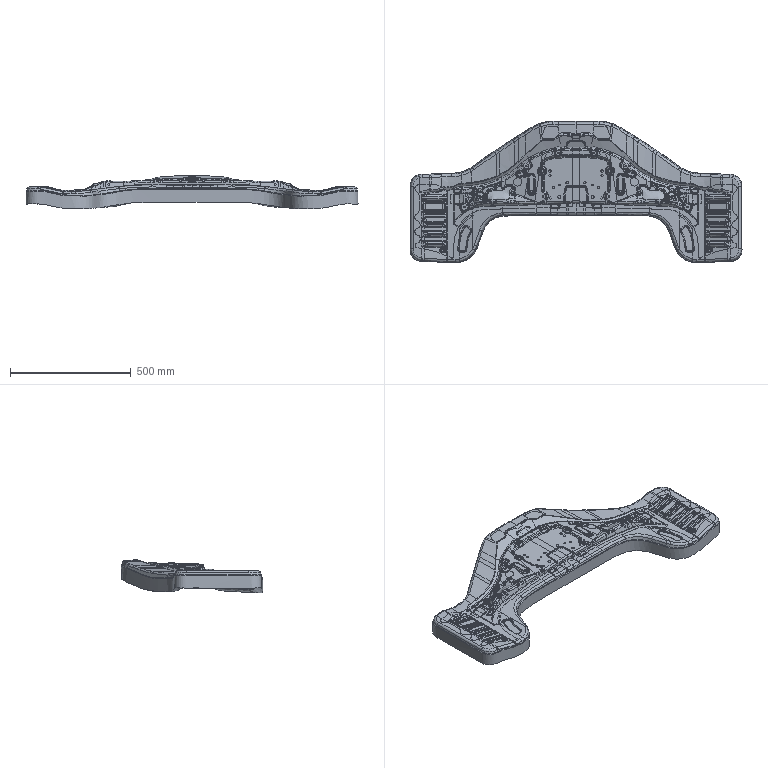Part | NX | features solid 2 | 1 solid | 2574 faces | box 1375 x 585.254 x 139.808 mm | volume 27699416 mm3 | spline 1466 | cylinder 694 | plane 385 | sphere 16 | cone 13 | commonest cylinder face diameters 9.6 x55 14.4 x52 8.4 x29 10.4 x27 7.6 x26 20 x20